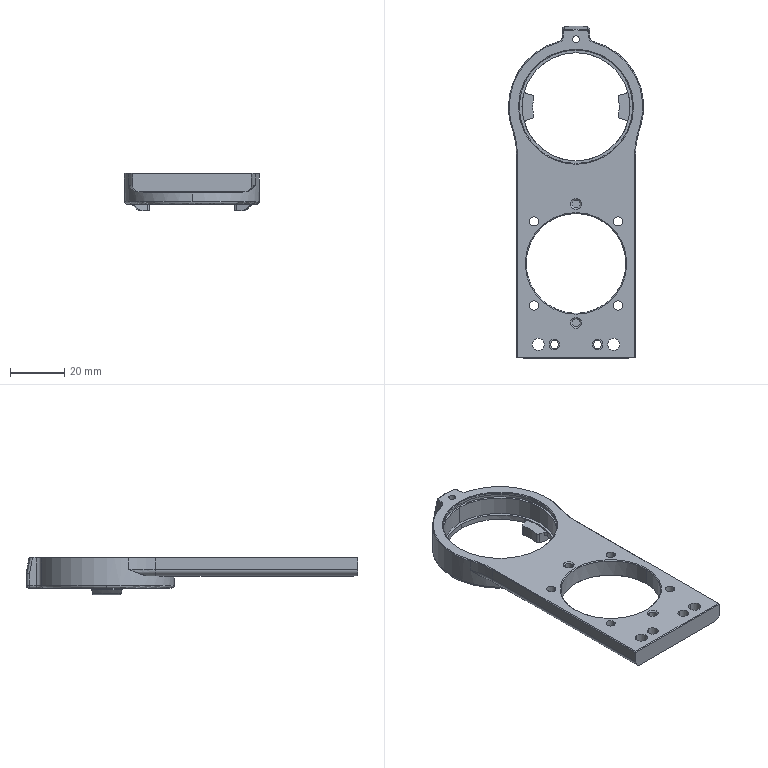Part | 1 solid | 218 faces | box 50 x 122.9 x 14 mm | volume 18666 mm3 | cylinder 105 | torus 42 | plane 41 | cone 20 | spline 8 | sphere 2 | commonest cylinder face diameters 2 x25 4 x24 3.4 x8 3 x4 3.02 x4 4.5 x4